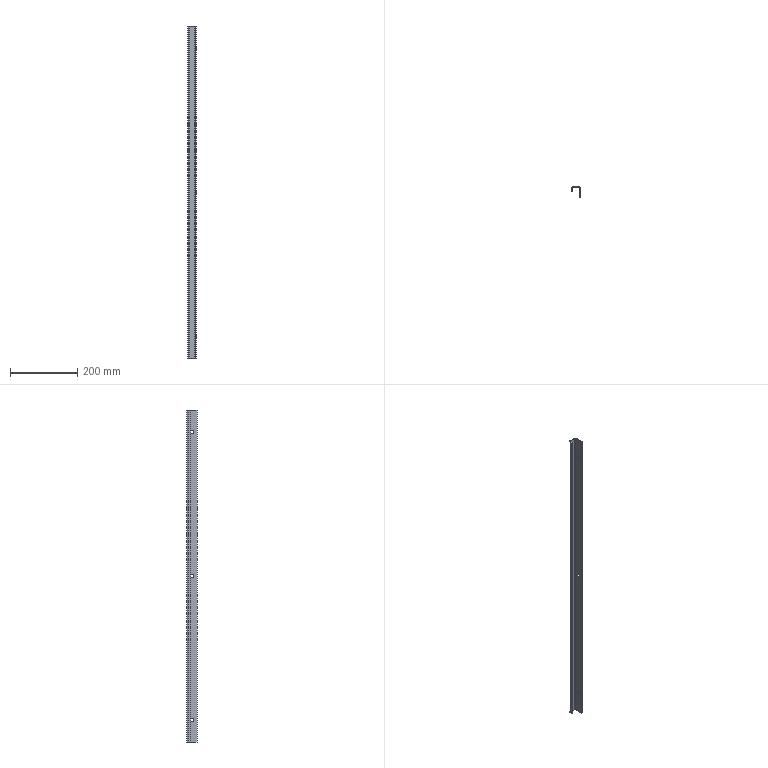Part | STEP file | 750078263 | 1 solid | 20 faces | box 25 x 30 x 985 mm | volume 118517 mm3 | cylinder 10 | plane 10 | commonest cylinder face diameters 10.5 x6 4 x2 8 x2
STEP:
#1=CARTESIAN_POINT('',(-2.,15.,432.75));
#2=VERTEX_POINT('',#1);
#3=CARTESIAN_POINT('',(-2.,15.,422.25));
#4=VERTEX_POINT('',#3);
#5=CARTESIAN_POINT('',(-2.,15.,427.5));
#6=DIRECTION('',(1.,0.,0.));
#7=DIRECTION('',(0.,0.,-1.));
#8=AXIS2_PLACEMENT_3D('',#5,#6,#7);
#9=CIRCLE('',#8,5.25);
#10=EDGE_CURVE('',#2,#4,#9,.T.);
#11=ORIENTED_EDGE('',*,*,#10,.F.);
#12=CARTESIAN_POINT('',(0.,15.,432.75));
#13=VERTEX_POINT('',#12);
#14=CARTESIAN_POINT('',(-2.,15.,432.75));
#15=DIRECTION('',(1.,0.,0.));
#16=VECTOR('',#15,1000.);
#17=LINE('',#14,#16);
#18=EDGE_CURVE('',#2,#13,#17,.T.);
#19=ORIENTED_EDGE('',*,*,#18,.T.);
#20=CARTESIAN_POINT('',(0.,15.,422.25));
#21=VERTEX_POINT('',#20);
#22=CARTESIAN_POINT('',(0.,15.,427.5));
#23=DIRECTION('',(-1.,0.,0.));
#24=DIRECTION('',(0.,0.,-1.));
#25=AXIS2_PLACEMENT_3D('',#22,#23,#24);
#26=CIRCLE('',#25,5.25);
#27=EDGE_CURVE('',#21,#13,#26,.T.);
#28=ORIENTED_EDGE('',*,*,#27,.F.);
#29=CARTESIAN_POINT('',(-2.,15.,422.25));
#30=DIRECTION('',(1.,0.,0.));
#31=VECTOR('',#30,1000.);
#32=LINE('',#29,#31);
#33=EDGE_CURVE('',#4,#21,#32,.T.);
#34=ORIENTED_EDGE('',*,*,#33,.F.);
#35=EDGE_LOOP('',(#11,#19,#28,#34));
#36=FACE_OUTER_BOUND('',#35,.T.);
#37=CARTESIAN_POINT('',(-2.,15.,427.5));
#38=DIRECTION('',(1.,0.,0.));
#39=DIRECTION('',(0.,0.,-1.));
#40=AXIS2_PLACEMENT_3D('',#37,#38,#39);
#41=CYLINDRICAL_SURFACE('',#40,5.25);
#42=ADVANCED_FACE('',(#36),#41,.F.);
#43=CARTESIAN_POINT('',(-2.,15.,5.25));
#44=VERTEX_POINT('',#43);
#45=CARTESIAN_POINT('',(-2.,15.,-5.25));
#46=VERTEX_POINT('',#45);
#47=CARTESIAN_POINT('',(-2.,15.,0.));
#48=DIRECTION('',(1.,0.,0.));
#49=DIRECTION('',(0.,0.,-1.));
#50=AXIS2_PLACEMENT_3D('',#47,#48,#49);
#51=CIRCLE('',#50,5.25);
#52=EDGE_CURVE('',#44,#46,#51,.T.);
#53=ORIENTED_EDGE('',*,*,#52,.F.);
#54=CARTESIAN_POINT('',(0.,15.,5.25));
#55=VERTEX_POINT('',#54);
#56=CARTESIAN_POINT('',(-2.,15.,5.25));
#57=DIRECTION('',(1.,0.,0.));
#58=VECTOR('',#57,1000.);
#59=LINE('',#56,#58);
#60=EDGE_CURVE('',#44,#55,#59,.T.);
#61=ORIENTED_EDGE('',*,*,#60,.T.);
#62=CARTESIAN_POINT('',(0.,15.,-5.25));
#63=VERTEX_POINT('',#62);
#64=CARTESIAN_POINT('',(0.,15.,0.));
#65=DIRECTION('',(-1.,0.,0.));
#66=DIRECTION('',(0.,0.,-1.));
#67=AXIS2_PLACEMENT_3D('',#64,#65,#66);
#68=CIRCLE('',#67,5.25);
#69=EDGE_CURVE('',#63,#55,#68,.T.);
#70=ORIENTED_EDGE('',*,*,#69,.F.);
#71=CARTESIAN_POINT('',(-2.,15.,-5.25));
#72=DIRECTION('',(1.,0.,0.));
#73=VECTOR('',#72,1000.);
#74=LINE('',#71,#73);
#75=EDGE_CURVE('',#46,#63,#74,.T.);
#76=ORIENTED_EDGE('',*,*,#75,.F.);
#77=EDGE_LOOP('',(#53,#61,#70,#76));
#78=FACE_OUTER_BOUND('',#77,.T.);
#79=CARTESIAN_POINT('',(-2.,15.,0.));
#80=DIRECTION('',(1.,0.,0.));
#81=DIRECTION('',(0.,0.,-1.));
#82=AXIS2_PLACEMENT_3D('',#79,#80,#81);
#83=CYLINDRICAL_SURFACE('',#82,5.25);
#84=ADVANCED_FACE('',(#78),#83,.F.);
#85=CARTESIAN_POINT('',(-2.,15.,-422.25));
#86=VERTEX_POINT('',#85);
#87=CARTESIAN_POINT('',(-2.,15.,-432.75));
#88=VERTEX_POINT('',#87);
#89=CARTESIAN_POINT('',(-2.,15.,-427.5));
#90=DIRECTION('',(1.,0.,0.));
#91=DIRECTION('',(0.,0.,-1.));
#92=AXIS2_PLACEMENT_3D('',#89,#90,#91);
#93=CIRCLE('',#92,5.25);
#94=EDGE_CURVE('',#86,#88,#93,.T.);
#95=ORIENTED_EDGE('',*,*,#94,.F.);
#96=CARTESIAN_POINT('',(0.,15.,-422.25));
#97=VERTEX_POINT('',#96);
#98=CARTESIAN_POINT('',(-2.,15.,-422.25));
#99=DIRECTION('',(1.,0.,0.));
#100=VECTOR('',#99,1000.);
#101=LINE('',#98,#100);
#102=EDGE_CURVE('',#86,#97,#101,.T.);
#103=ORIENTED_EDGE('',*,*,#102,.T.);
#104=CARTESIAN_POINT('',(0.,15.,-432.75));
#105=VERTEX_POINT('',#104);
#106=CARTESIAN_POINT('',(0.,15.,-427.5));
#107=DIRECTION('',(-1.,0.,0.));
#108=DIRECTION('',(0.,0.,-1.));
#109=AXIS2_PLACEMENT_3D('',#106,#107,#108);
#110=CIRCLE('',#109,5.25);
#111=EDGE_CURVE('',#105,#97,#110,.T.);
#112=ORIENTED_EDGE('',*,*,#111,.F.);
#113=CARTESIAN_POINT('',(-2.,15.,-432.75));
#114=DIRECTION('',(1.,0.,0.));
#115=VECTOR('',#114,1000.);
#116=LINE('',#113,#115);
#117=EDGE_CURVE('',#88,#105,#116,.T.);
#118=ORIENTED_EDGE('',*,*,#117,.F.);
#119=EDGE_LOOP('',(#95,#103,#112,#118));
#120=FACE_OUTER_BOUND('',#119,.T.);
#121=CARTESIAN_POINT('',(-2.,15.,-427.5));
#122=DIRECTION('',(1.,0.,0.));
#123=DIRECTION('',(0.,0.,-1.));
#124=AXIS2_PLACEMENT_3D('',#121,#122,#123);
#125=CYLINDRICAL_SURFACE('',#124,5.25);
#126=ADVANCED_FACE('',(#120),#125,.F.);
#127=CARTESIAN_POINT('',(0.,26.,492.5));
#128=VERTEX_POINT('',#127);
#129=CARTESIAN_POINT('',(0.,0.,492.5));
#130=VERTEX_POINT('',#129);
#131=CARTESIAN_POINT('',(0.,30.,492.5));
#132=DIRECTION('',(0.,-1.,0.));
#133=VECTOR('',#132,1000.);
#134=LINE('',#131,#133);
#135=EDGE_CURVE('',#128,#130,#134,.T.);
#136=ORIENTED_EDGE('',*,*,#135,.T.);
#137=CARTESIAN_POINT('',(0.,0.,-492.5));
#138=VERTEX_POINT('',#137);
#139=CARTESIAN_POINT('',(0.,0.,492.5));
#140=DIRECTION('',(0.,0.,-1.));
#141=VECTOR('',#140,1000.);
#142=LINE('',#139,#141);
#143=EDGE_CURVE('',#130,#138,#142,.T.);
#144=ORIENTED_EDGE('',*,*,#143,.T.);
#145=CARTESIAN_POINT('',(0.,26.,-492.5));
#146=VERTEX_POINT('',#145);
#147=CARTESIAN_POINT('',(0.,30.,-492.5));
#148=DIRECTION('',(0.,1.,0.));
#149=VECTOR('',#148,1000.);
#150=LINE('',#147,#149);
#151=EDGE_CURVE('',#138,#146,#150,.T.);
#152=ORIENTED_EDGE('',*,*,#151,.T.);
#153=CARTESIAN_POINT('',(0.,26.,492.5));
#154=DIRECTION('',(0.,0.,1.));
#155=VECTOR('',#154,1000.);
#156=LINE('',#153,#155);
#157=EDGE_CURVE('',#146,#128,#156,.T.);
#158=ORIENTED_EDGE('',*,*,#157,.T.);
#159=EDGE_LOOP('',(#136,#144,#152,#158));
#160=FACE_OUTER_BOUND('',#159,.T.);
#161=ORIENTED_EDGE('',*,*,#27,.T.);
#162=CARTESIAN_POINT('',(0.,15.,427.5));
#163=DIRECTION('',(-1.,0.,0.));
#164=DIRECTION('',(0.,0.,-1.));
#165=AXIS2_PLACEMENT_3D('',#162,#163,#164);
#166=CIRCLE('',#165,5.25);
#167=EDGE_CURVE('',#13,#21,#166,.T.);
#168=ORIENTED_EDGE('',*,*,#167,.T.);
#169=EDGE_LOOP('',(#161,#168));
#170=FACE_BOUND('',#169,.T.);
#171=ORIENTED_EDGE('',*,*,#69,.T.);
#172=CARTESIAN_POINT('',(0.,15.,0.));
#173=DIRECTION('',(-1.,0.,0.));
#174=DIRECTION('',(0.,0.,-1.));
#175=AXIS2_PLACEMENT_3D('',#172,#173,#174);
#176=CIRCLE('',#175,5.25);
#177=EDGE_CURVE('',#55,#63,#176,.T.);
#178=ORIENTED_EDGE('',*,*,#177,.T.);
#179=EDGE_LOOP('',(#171,#178));
#180=FACE_BOUND('',#179,.T.);
#181=ORIENTED_EDGE('',*,*,#111,.T.);
#182=CARTESIAN_POINT('',(0.,15.,-427.5));
#183=DIRECTION('',(-1.,0.,0.));
#184=DIRECTION('',(0.,0.,-1.));
#185=AXIS2_PLACEMENT_3D('',#182,#183,#184);
#186=CIRCLE('',#185,5.25);
#187=EDGE_CURVE('',#97,#105,#186,.T.);
#188=ORIENTED_EDGE('',*,*,#187,.T.);
#189=EDGE_LOOP('',(#181,#188));
#190=FACE_BOUND('',#189,.T.);
#191=CARTESIAN_POINT('',(0.,30.,492.5));
#192=DIRECTION('',(1.,0.,0.));
#193=DIRECTION('',(0.,0.,-1.));
#194=AXIS2_PLACEMENT_3D('',#191,#192,#193);
#195=PLANE('',#194);
#196=ADVANCED_FACE('',(#160,#170,#180,#190),#195,.T.);
#197=CARTESIAN_POINT('',(-2.,0.,-492.5));
#198=VERTEX_POINT('',#197);
#199=CARTESIAN_POINT('',(0.,0.,-492.5));
#200=DIRECTION('',(1.,0.,0.));
#201=VECTOR('',#200,1000.);
#202=LINE('',#199,#201);
#203=EDGE_CURVE('',#198,#138,#202,.T.);
#204=ORIENTED_EDGE('',*,*,#203,.T.);
#205=ORIENTED_EDGE('',*,*,#143,.F.);
#206=CARTESIAN_POINT('',(-2.,0.,492.5));
#207=VERTEX_POINT('',#206);
#208=CARTESIAN_POINT('',(0.,0.,492.5));
#209=DIRECTION('',(-1.,0.,0.));
#210=VECTOR('',#209,1000.);
#211=LINE('',#208,#210);
#212=EDGE_CURVE('',#130,#207,#211,.T.);
#213=ORIENTED_EDGE('',*,*,#212,.T.);
#214=CARTESIAN_POINT('',(-2.,0.,492.5));
#215=DIRECTION('',(0.,0.,-1.));
#216=VECTOR('',#215,1000.);
#217=LINE('',#214,#216);
#218=EDGE_CURVE('',#207,#198,#217,.T.);
#219=ORIENTED_EDGE('',*,*,#218,.T.);
#220=EDGE_LOOP('',(#204,#205,#213,#219));
#221=FACE_OUTER_BOUND('',#220,.T.);
#222=CARTESIAN_POINT('',(0.,0.,492.5));
#223=DIRECTION('',(0.,-1.,0.));
#224=DIRECTION('',(0.,0.,-1.));
#225=AXIS2_PLACEMENT_3D('',#222,#223,#224);
#226=PLANE('',#225);
#227=ADVANCED_FACE('',(#221),#226,.T.);
#228=CARTESIAN_POINT('',(-2.,26.,492.5));
#229=VERTEX_POINT('',#228);
#230=CARTESIAN_POINT('',(-2.,30.,492.5));
#231=DIRECTION('',(0.,-1.,0.));
#232=VECTOR('',#231,1000.);
#233=LINE('',#230,#232);
#234=EDGE_CURVE('',#229,#207,#233,.T.);
#235=ORIENTED_EDGE('',*,*,#234,.T.);
#236=ORIENTED_EDGE('',*,*,#212,.F.);
#237=ORIENTED_EDGE('',*,*,#135,.F.);
#238=CARTESIAN_POINT('',(-4.,30.,492.5));
#239=VERTEX_POINT('',#238);
#240=CARTESIAN_POINT('',(-4.,26.,492.5));
#241=DIRECTION('',(0.,0.,1.));
#242=DIRECTION('',(-1.,0.,0.));
#243=AXIS2_PLACEMENT_3D('',#240,#241,#242);
#244=CIRCLE('',#243,4.);
#245=EDGE_CURVE('',#128,#239,#244,.T.);
#246=ORIENTED_EDGE('',*,*,#245,.T.);
#247=CARTESIAN_POINT('',(-21.,30.,492.5));
#248=VERTEX_POINT('',#247);
#249=CARTESIAN_POINT('',(0.,30.,492.5));
#250=DIRECTION('',(-1.,0.,0.));
#251=VECTOR('',#250,1000.);
#252=LINE('',#249,#251);
#253=EDGE_CURVE('',#239,#248,#252,.T.);
#254=ORIENTED_EDGE('',*,*,#253,.T.);
#255=CARTESIAN_POINT('',(-25.,26.,492.5));
#256=VERTEX_POINT('',#255);
#257=CARTESIAN_POINT('',(-21.,26.,492.5));
#258=DIRECTION('',(0.,0.,1.));
#259=DIRECTION('',(-1.,0.,0.));
#260=AXIS2_PLACEMENT_3D('',#257,#258,#259);
#261=CIRCLE('',#260,4.);
#262=EDGE_CURVE('',#248,#256,#261,.T.);
#263=ORIENTED_EDGE('',*,*,#262,.T.);
#264=CARTESIAN_POINT('',(-25.,18.,492.5));
#265=VERTEX_POINT('',#264);
#266=CARTESIAN_POINT('',(-25.,30.,492.5));
#267=DIRECTION('',(0.,-1.,0.));
#268=VECTOR('',#267,1000.);
#269=LINE('',#266,#268);
#270=EDGE_CURVE('',#256,#265,#269,.T.);
#271=ORIENTED_EDGE('',*,*,#270,.T.);
#272=CARTESIAN_POINT('',(-23.,18.,492.5));
#273=VERTEX_POINT('',#272);
#274=CARTESIAN_POINT('',(0.,18.,492.5));
#275=DIRECTION('',(1.,0.,0.));
#276=VECTOR('',#275,1000.);
#277=LINE('',#274,#276);
#278=EDGE_CURVE('',#265,#273,#277,.T.);
#279=ORIENTED_EDGE('',*,*,#278,.T.);
#280=CARTESIAN_POINT('',(-23.,26.,492.5));
#281=VERTEX_POINT('',#280);
#282=CARTESIAN_POINT('',(-23.,30.,492.5));
#283=DIRECTION('',(0.,1.,0.));
#284=VECTOR('',#283,1000.);
#285=LINE('',#282,#284);
#286=EDGE_CURVE('',#273,#281,#285,.T.);
#287=ORIENTED_EDGE('',*,*,#286,.T.);
#288=CARTESIAN_POINT('',(-21.,28.,492.5));
#289=VERTEX_POINT('',#288);
#290=CARTESIAN_POINT('',(-21.,26.,492.5));
#291=DIRECTION('',(0.,0.,-1.));
#292=DIRECTION('',(-1.,0.,0.));
#293=AXIS2_PLACEMENT_3D('',#290,#291,#292);
#294=CIRCLE('',#293,2.);
#295=EDGE_CURVE('',#281,#289,#294,.T.);
#296=ORIENTED_EDGE('',*,*,#295,.T.);
#297=CARTESIAN_POINT('',(-4.,28.,492.5));
#298=VERTEX_POINT('',#297);
#299=CARTESIAN_POINT('',(0.,28.,492.5));
#300=DIRECTION('',(1.,0.,0.));
#301=VECTOR('',#300,1000.);
#302=LINE('',#299,#301);
#303=EDGE_CURVE('',#289,#298,#302,.T.);
#304=ORIENTED_EDGE('',*,*,#303,.T.);
#305=CARTESIAN_POINT('',(-4.,26.,492.5));
#306=DIRECTION('',(0.,0.,-1.));
#307=DIRECTION('',(-1.,0.,0.));
#308=AXIS2_PLACEMENT_3D('',#305,#306,#307);
#309=CIRCLE('',#308,2.);
#310=EDGE_CURVE('',#298,#229,#309,.T.);
#311=ORIENTED_EDGE('',*,*,#310,.T.);
#312=EDGE_LOOP('',(#235,#236,#237,#246,#254,#263,#271,#279,#287,#296,#304,#311));
#313=FACE_OUTER_BOUND('',#312,.T.);
#314=CARTESIAN_POINT('',(0.,30.,492.5));
#315=DIRECTION('',(0.,0.,1.));
#316=DIRECTION('',(1.,0.,0.));
#317=AXIS2_PLACEMENT_3D('',#314,#315,#316);
#318=PLANE('',#317);
#319=ADVANCED_FACE('',(#313),#318,.T.);
#320=ORIENTED_EDGE('',*,*,#245,.F.);
#321=ORIENTED_EDGE('',*,*,#157,.F.);
#322=CARTESIAN_POINT('',(-4.,30.,-492.5));
#323=VERTEX_POINT('',#322);
#324=CARTESIAN_POINT('',(-4.,26.,-492.5));
#325=DIRECTION('',(0.,0.,1.));
#326=DIRECTION('',(-1.,0.,0.));
#327=AXIS2_PLACEMENT_3D('',#324,#325,#326);
#328=CIRCLE('',#327,4.);
#329=EDGE_CURVE('',#146,#323,#328,.T.);
#330=ORIENTED_EDGE('',*,*,#329,.T.);
#331=CARTESIAN_POINT('',(-4.,30.,492.5));
#332=DIRECTION('',(0.,0.,1.));
#333=VECTOR('',#332,1000.);
#334=LINE('',#331,#333);
#335=EDGE_CURVE('',#323,#239,#334,.T.);
#336=ORIENTED_EDGE('',*,*,#335,.T.);
#337=EDGE_LOOP('',(#320,#321,#330,#336));
#338=FACE_OUTER_BOUND('',#337,.T.);
#339=CARTESIAN_POINT('',(-4.,26.,492.5));
#340=DIRECTION('',(0.,0.,-1.));
#341=DIRECTION('',(-1.,0.,0.));
#342=AXIS2_PLACEMENT_3D('',#339,#340,#341);
#343=CYLINDRICAL_SURFACE('',#342,4.);
#344=ADVANCED_FACE('',(#338),#343,.T.);
#345=CARTESIAN_POINT('',(-21.,30.,-492.5));
#346=VERTEX_POINT('',#345);
#347=CARTESIAN_POINT('',(-25.,26.,-492.5));
#348=VERTEX_POINT('',#347);
#349=CARTESIAN_POINT('',(-21.,26.,-492.5));
#350=DIRECTION('',(0.,0.,1.));
#351=DIRECTION('',(-1.,0.,0.));
#352=AXIS2_PLACEMENT_3D('',#349,#350,#351);
#353=CIRCLE('',#352,4.);
#354=EDGE_CURVE('',#346,#348,#353,.T.);
#355=ORIENTED_EDGE('',*,*,#354,.F.);
#356=CARTESIAN_POINT('',(-25.,30.,-492.5));
#357=DIRECTION('',(-1.,0.,0.));
#358=VECTOR('',#357,1000.);
#359=LINE('',#356,#358);
#360=EDGE_CURVE('',#323,#346,#359,.T.);
#361=ORIENTED_EDGE('',*,*,#360,.F.);
#362=ORIENTED_EDGE('',*,*,#329,.F.);
#363=ORIENTED_EDGE('',*,*,#151,.F.);
#364=ORIENTED_EDGE('',*,*,#203,.F.);
#365=CARTESIAN_POINT('',(-2.,26.,-492.5));
#366=VERTEX_POINT('',#365);
#367=CARTESIAN_POINT('',(-2.,18.,-492.5));
#368=DIRECTION('',(0.,-1.,0.));
#369=VECTOR('',#368,1000.);
#370=LINE('',#367,#369);
#371=EDGE_CURVE('',#366,#198,#370,.T.);
#372=ORIENTED_EDGE('',*,*,#371,.F.);
#373=CARTESIAN_POINT('',(-4.,28.,-492.5));
#374=VERTEX_POINT('',#373);
#375=CARTESIAN_POINT('',(-4.,26.,-492.5));
#376=DIRECTION('',(0.,0.,-1.));
#377=DIRECTION('',(-1.,0.,0.));
#378=AXIS2_PLACEMENT_3D('',#375,#376,#377);
#379=CIRCLE('',#378,2.);
#380=EDGE_CURVE('',#374,#366,#379,.T.);
#381=ORIENTED_EDGE('',*,*,#380,.F.);
#382=CARTESIAN_POINT('',(-21.,28.,-492.5));
#383=VERTEX_POINT('',#382);
#384=CARTESIAN_POINT('',(-25.,28.,-492.5));
#385=DIRECTION('',(1.,0.,0.));
#386=VECTOR('',#385,1000.);
#387=LINE('',#384,#386);
#388=EDGE_CURVE('',#383,#374,#387,.T.);
#389=ORIENTED_EDGE('',*,*,#388,.F.);
#390=CARTESIAN_POINT('',(-23.,26.,-492.5));
#391=VERTEX_POINT('',#390);
#392=CARTESIAN_POINT('',(-21.,26.,-492.5));
#393=DIRECTION('',(0.,0.,-1.));
#394=DIRECTION('',(-1.,0.,0.));
#395=AXIS2_PLACEMENT_3D('',#392,#393,#394);
#396=CIRCLE('',#395,2.);
#397=EDGE_CURVE('',#391,#383,#396,.T.);
#398=ORIENTED_EDGE('',*,*,#397,.F.);
#399=CARTESIAN_POINT('',(-23.,18.,-492.5));
#400=VERTEX_POINT('',#399);
#401=CARTESIAN_POINT('',(-23.,18.,-492.5));
#402=DIRECTION('',(0.,1.,0.));
#403=VECTOR('',#402,1000.);
#404=LINE('',#401,#403);
#405=EDGE_CURVE('',#400,#391,#404,.T.);
#406=ORIENTED_EDGE('',*,*,#405,.F.);
#407=CARTESIAN_POINT('',(-25.,18.,-492.5));
#408=VERTEX_POINT('',#407);
#409=CARTESIAN_POINT('',(-25.,18.,-492.5));
#410=DIRECTION('',(1.,0.,0.));
#411=VECTOR('',#410,1000.);
#412=LINE('',#409,#411);
#413=EDGE_CURVE('',#408,#400,#412,.T.);
#414=ORIENTED_EDGE('',*,*,#413,.F.);
#415=CARTESIAN_POINT('',(-25.,18.,-492.5));
#416=DIRECTION('',(0.,-1.,0.));
#417=VECTOR('',#416,1000.);
#418=LINE('',#415,#417);
#419=EDGE_CURVE('',#348,#408,#418,.T.);
#420=ORIENTED_EDGE('',*,*,#419,.F.);
#421=EDGE_LOOP('',(#355,#361,#362,#363,#364,#372,#381,#389,#398,#406,#414,#420));
#422=FACE_OUTER_BOUND('',#421,.T.);
#423=CARTESIAN_POINT('',(-25.,18.,-492.5));
#424=DIRECTION('',(0.,0.,1.));
#425=DIRECTION('',(1.,0.,0.));
#426=AXIS2_PLACEMENT_3D('',#423,#424,#425);
#427=PLANE('',#426);
#428=ADVANCED_FACE('',(#422),#427,.F.);
#429=ORIENTED_EDGE('',*,*,#18,.F.);
#430=CARTESIAN_POINT('',(-2.,15.,427.5));
#431=DIRECTION('',(1.,0.,0.));
#432=DIRECTION('',(0.,0.,-1.));
#433=AXIS2_PLACEMENT_3D('',#430,#431,#432);
#434=CIRCLE('',#433,5.25);
#435=EDGE_CURVE('',#4,#2,#434,.T.);
#436=ORIENTED_EDGE('',*,*,#435,.F.);
#437=ORIENTED_EDGE('',*,*,#33,.T.);
#438=ORIENTED_EDGE('',*,*,#167,.F.);
#439=EDGE_LOOP('',(#429,#436,#437,#438));
#440=FACE_OUTER_BOUND('',#439,.T.);
#441=CARTESIAN_POINT('',(-2.,15.,427.5));
#442=DIRECTION('',(1.,0.,0.));
#443=DIRECTION('',(0.,0.,-1.));
#444=AXIS2_PLACEMENT_3D('',#441,#442,#443);
#445=CYLINDRICAL_SURFACE('',#444,5.25);
#446=ADVANCED_FACE('',(#440),#445,.F.);
#447=ORIENTED_EDGE('',*,*,#60,.F.);
#448=CARTESIAN_POINT('',(-2.,15.,0.));
#449=DIRECTION('',(1.,0.,0.));
#450=DIRECTION('',(0.,0.,-1.));
#451=AXIS2_PLACEMENT_3D('',#448,#449,#450);
#452=CIRCLE('',#451,5.25);
#453=EDGE_CURVE('',#46,#44,#452,.T.);
#454=ORIENTED_EDGE('',*,*,#453,.F.);
#455=ORIENTED_EDGE('',*,*,#75,.T.);
#456=ORIENTED_EDGE('',*,*,#177,.F.);
#457=EDGE_LOOP('',(#447,#454,#455,#456));
#458=FACE_OUTER_BOUND('',#457,.T.);
#459=CARTESIAN_POINT('',(-2.,15.,0.));
#460=DIRECTION('',(1.,0.,0.));
#461=DIRECTION('',(0.,0.,-1.));
#462=AXIS2_PLACEMENT_3D('',#459,#460,#461);
#463=CYLINDRICAL_SURFACE('',#462,5.25);
#464=ADVANCED_FACE('',(#458),#463,.F.);
#465=ORIENTED_EDGE('',*,*,#102,.F.);
#466=CARTESIAN_POINT('',(-2.,15.,-427.5));
#467=DIRECTION('',(1.,0.,0.));
#468=DIRECTION('',(0.,0.,-1.));
#469=AXIS2_PLACEMENT_3D('',#466,#467,#468);
#470=CIRCLE('',#469,5.25);
#471=EDGE_CURVE('',#88,#86,#470,.T.);
#472=ORIENTED_EDGE('',*,*,#471,.F.);
#473=ORIENTED_EDGE('',*,*,#117,.T.);
#474=ORIENTED_EDGE('',*,*,#187,.F.);
#475=EDGE_LOOP('',(#465,#472,#473,#474));
#476=FACE_OUTER_BOUND('',#475,.T.);
#477=CARTESIAN_POINT('',(-2.,15.,-427.5));
#478=DIRECTION('',(1.,0.,0.));
#479=DIRECTION('',(0.,0.,-1.));
#480=AXIS2_PLACEMENT_3D('',#477,#478,#479);
#481=CYLINDRICAL_SURFACE('',#480,5.25);
#482=ADVANCED_FACE('',(#476),#481,.F.);
#483=ORIENTED_EDGE('',*,*,#218,.F.);
#484=ORIENTED_EDGE('',*,*,#234,.F.);
#485=CARTESIAN_POINT('',(-2.,26.,492.5));
#486=DIRECTION('',(0.,0.,1.));
#487=VECTOR('',#486,1000.);
#488=LINE('',#485,#487);
#489=EDGE_CURVE('',#366,#229,#488,.T.);
#490=ORIENTED_EDGE('',*,*,#489,.F.);
#491=ORIENTED_EDGE('',*,*,#371,.T.);
#492=EDGE_LOOP('',(#483,#484,#490,#491));
#493=FACE_OUTER_BOUND('',#492,.T.);
#494=ORIENTED_EDGE('',*,*,#435,.T.);
#495=ORIENTED_EDGE('',*,*,#10,.T.);
#496=EDGE_LOOP('',(#494,#495));
#497=FACE_BOUND('',#496,.T.);
#498=ORIENTED_EDGE('',*,*,#453,.T.);
#499=ORIENTED_EDGE('',*,*,#52,.T.);
#500=EDGE_LOOP('',(#498,#499));
#501=FACE_BOUND('',#500,.T.);
#502=ORIENTED_EDGE('',*,*,#471,.T.);
#503=ORIENTED_EDGE('',*,*,#94,.T.);
#504=EDGE_LOOP('',(#502,#503));
#505=FACE_BOUND('',#504,.T.);
#506=CARTESIAN_POINT('',(-2.,30.,492.5));
#507=DIRECTION('',(1.,0.,0.));
#508=DIRECTION('',(0.,0.,-1.));
#509=AXIS2_PLACEMENT_3D('',#506,#507,#508);
#510=PLANE('',#509);
#511=ADVANCED_FACE('',(#493,#497,#501,#505),#510,.F.);
#512=ORIENTED_EDGE('',*,*,#489,.T.);
#513=ORIENTED_EDGE('',*,*,#310,.F.);
#514=CARTESIAN_POINT('',(-4.,28.,492.5));
#515=DIRECTION('',(0.,0.,1.));
#516=VECTOR('',#515,1000.);
#517=LINE('',#514,#516);
#518=EDGE_CURVE('',#374,#298,#517,.T.);
#519=ORIENTED_EDGE('',*,*,#518,.F.);
#520=ORIENTED_EDGE('',*,*,#380,.T.);
#521=EDGE_LOOP('',(#512,#513,#519,#520));
#522=FACE_OUTER_BOUND('',#521,.T.);
#523=CARTESIAN_POINT('',(-4.,26.,492.5));
#524=DIRECTION('',(0.,0.,-1.));
#525=DIRECTION('',(-1.,0.,0.));
#526=AXIS2_PLACEMENT_3D('',#523,#524,#525);
#527=CYLINDRICAL_SURFACE('',#526,2.);
#528=ADVANCED_FACE('',(#522),#527,.F.);
#529=ORIENTED_EDGE('',*,*,#518,.T.);
#530=ORIENTED_EDGE('',*,*,#303,.F.);
#531=CARTESIAN_POINT('',(-21.,28.,492.5));
#532=DIRECTION('',(0.,0.,1.));
#533=VECTOR('',#532,1000.);
#534=LINE('',#531,#533);
#535=EDGE_CURVE('',#383,#289,#534,.T.);
#536=ORIENTED_EDGE('',*,*,#535,.F.);
#537=ORIENTED_EDGE('',*,*,#388,.T.);
#538=EDGE_LOOP('',(#529,#530,#536,#537));
#539=FACE_OUTER_BOUND('',#538,.T.);
#540=CARTESIAN_POINT('',(-25.,28.,492.5));
#541=DIRECTION('',(0.,1.,0.));
#542=DIRECTION('',(0.,0.,1.));
#543=AXIS2_PLACEMENT_3D('',#540,#541,#542);
#544=PLANE('',#543);
#545=ADVANCED_FACE('',(#539),#544,.F.);
#546=ORIENTED_EDGE('',*,*,#535,.T.);
#547=ORIENTED_EDGE('',*,*,#295,.F.);
#548=CARTESIAN_POINT('',(-23.,26.,492.5));
#549=DIRECTION('',(0.,0.,1.));
#550=VECTOR('',#549,1000.);
#551=LINE('',#548,#550);
#552=EDGE_CURVE('',#391,#281,#551,.T.);
#553=ORIENTED_EDGE('',*,*,#552,.F.);
#554=ORIENTED_EDGE('',*,*,#397,.T.);
#555=EDGE_LOOP('',(#546,#547,#553,#554));
#556=FACE_OUTER_BOUND('',#555,.T.);
#557=CARTESIAN_POINT('',(-21.,26.,492.5));
#558=DIRECTION('',(0.,0.,-1.));
#559=DIRECTION('',(-1.,0.,0.));
#560=AXIS2_PLACEMENT_3D('',#557,#558,#559);
#561=CYLINDRICAL_SURFACE('',#560,2.);
#562=ADVANCED_FACE('',(#556),#561,.F.);
#563=ORIENTED_EDGE('',*,*,#552,.T.);
#564=ORIENTED_EDGE('',*,*,#286,.F.);
#565=CARTESIAN_POINT('',(-23.,18.,492.5));
#566=DIRECTION('',(0.,0.,1.));
#567=VECTOR('',#566,1000.);
#568=LINE('',#565,#567);
#569=EDGE_CURVE('',#400,#273,#568,.T.);
#570=ORIENTED_EDGE('',*,*,#569,.F.);
#571=ORIENTED_EDGE('',*,*,#405,.T.);
#572=EDGE_LOOP('',(#563,#564,#570,#571));
#573=FACE_OUTER_BOUND('',#572,.T.);
#574=CARTESIAN_POINT('',(-23.,18.,492.5));
#575=DIRECTION('',(-1.,0.,0.));
#576=DIRECTION('',(0.,0.,1.));
#577=AXIS2_PLACEMENT_3D('',#574,#575,#576);
#578=PLANE('',#577);
#579=ADVANCED_FACE('',(#573),#578,.F.);
#580=ORIENTED_EDGE('',*,*,#278,.F.);
#581=CARTESIAN_POINT('',(-25.,18.,492.5));
#582=DIRECTION('',(0.,0.,1.));
#583=VECTOR('',#582,1000.);
#584=LINE('',#581,#583);
#585=EDGE_CURVE('',#408,#265,#584,.T.);
#586=ORIENTED_EDGE('',*,*,#585,.F.);
#587=ORIENTED_EDGE('',*,*,#413,.T.);
#588=ORIENTED_EDGE('',*,*,#569,.T.);
#589=EDGE_LOOP('',(#580,#586,#587,#588));
#590=FACE_OUTER_BOUND('',#589,.T.);
#591=CARTESIAN_POINT('',(-25.,18.,492.5));
#592=DIRECTION('',(0.,1.,0.));
#593=DIRECTION('',(0.,0.,1.));
#594=AXIS2_PLACEMENT_3D('',#591,#592,#593);
#595=PLANE('',#594);
#596=ADVANCED_FACE('',(#590),#595,.F.);
#597=ORIENTED_EDGE('',*,*,#270,.F.);
#598=CARTESIAN_POINT('',(-25.,26.,492.5));
#599=DIRECTION('',(0.,0.,-1.));
#600=VECTOR('',#599,1000.);
#601=LINE('',#598,#600);
#602=EDGE_CURVE('',#256,#348,#601,.T.);
#603=ORIENTED_EDGE('',*,*,#602,.T.);
#604=ORIENTED_EDGE('',*,*,#419,.T.);
#605=ORIENTED_EDGE('',*,*,#585,.T.);
#606=EDGE_LOOP('',(#597,#603,#604,#605));
#607=FACE_OUTER_BOUND('',#606,.T.);
#608=CARTESIAN_POINT('',(-25.,18.,492.5));
#609=DIRECTION('',(-1.,0.,0.));
#610=DIRECTION('',(0.,0.,1.));
#611=AXIS2_PLACEMENT_3D('',#608,#609,#610);
#612=PLANE('',#611);
#613=ADVANCED_FACE('',(#607),#612,.T.);
#614=ORIENTED_EDGE('',*,*,#262,.F.);
#615=CARTESIAN_POINT('',(-21.,30.,492.5));
#616=DIRECTION('',(0.,0.,-1.));
#617=VECTOR('',#616,1000.);
#618=LINE('',#615,#617);
#619=EDGE_CURVE('',#248,#346,#618,.T.);
#620=ORIENTED_EDGE('',*,*,#619,.T.);
#621=ORIENTED_EDGE('',*,*,#354,.T.);
#622=ORIENTED_EDGE('',*,*,#602,.F.);
#623=EDGE_LOOP('',(#614,#620,#621,#622));
#624=FACE_OUTER_BOUND('',#623,.T.);
#625=CARTESIAN_POINT('',(-21.,26.,492.5));
#626=DIRECTION('',(0.,0.,-1.));
#627=DIRECTION('',(-1.,0.,0.));
#628=AXIS2_PLACEMENT_3D('',#625,#626,#627);
#629=CYLINDRICAL_SURFACE('',#628,4.);
#630=ADVANCED_FACE('',(#624),#629,.T.);
#631=ORIENTED_EDGE('',*,*,#253,.F.);
#632=ORIENTED_EDGE('',*,*,#335,.F.);
#633=ORIENTED_EDGE('',*,*,#360,.T.);
#634=ORIENTED_EDGE('',*,*,#619,.F.);
#635=EDGE_LOOP('',(#631,#632,#633,#634));
#636=FACE_OUTER_BOUND('',#635,.T.);
#637=CARTESIAN_POINT('',(-25.,30.,492.5));
#638=DIRECTION('',(0.,1.,0.));
#639=DIRECTION('',(0.,0.,1.));
#640=AXIS2_PLACEMENT_3D('',#637,#638,#639);
#641=PLANE('',#640);
#642=ADVANCED_FACE('',(#636),#641,.T.);
#643=CLOSED_SHELL('',(#42,#84,#126,#196,#227,#319,#344,#428,#446,#464,#482,#511,#528,#545,#562,#579,#596,#613,#630,#642));
#644=MANIFOLD_SOLID_BREP('',#643);
#645=CARTESIAN_POINT('',(0.,0.,0.));
#646=DIRECTION('',(0.,0.,1.));
#647=DIRECTION('',(1.,0.,0.));
#648=AXIS2_PLACEMENT_3D('',#645,#646,#647);
#649=(LENGTH_UNIT()NAMED_UNIT(*)SI_UNIT(.MILLI.,.METRE.));
#650=UNCERTAINTY_MEASURE_WITH_UNIT(LENGTH_MEASURE(0.00001),#649,'','');
#651=(NAMED_UNIT(*)PLANE_ANGLE_UNIT()SI_UNIT($,.RADIAN.));
#652=(NAMED_UNIT(*)SI_UNIT($,.STERADIAN.)SOLID_ANGLE_UNIT());
#653=(GEOMETRIC_REPRESENTATION_CONTEXT(3)GLOBAL_UNCERTAINTY_ASSIGNED_CONTEXT((#650))GLOBAL_UNIT_ASSIGNED_CONTEXT((#649,#651,#652))REPRESENTATION_CONTEXT('',''));
#654=ADVANCED_BREP_SHAPE_REPRESENTATION('',(#644,#648),#653);